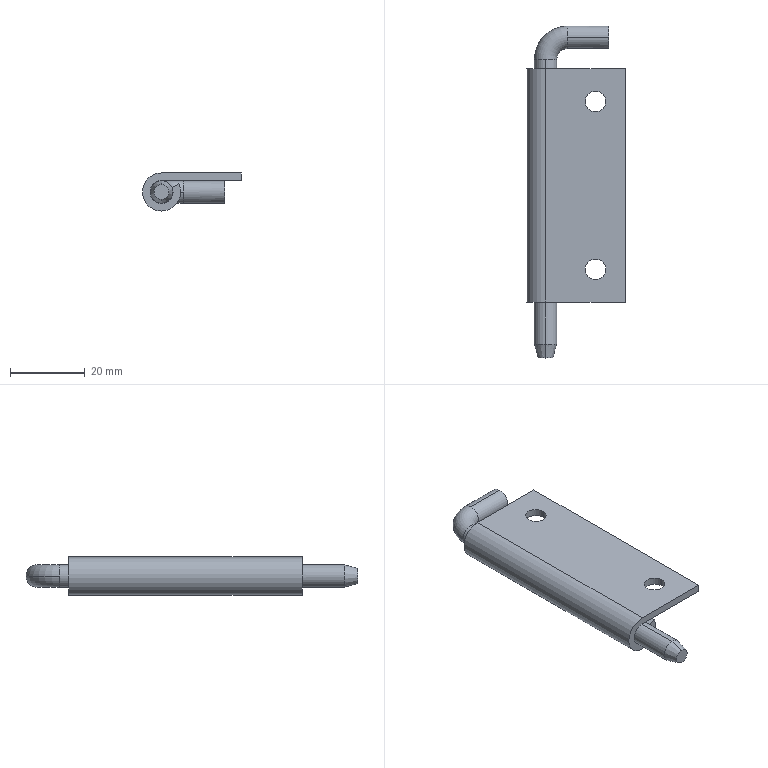Part | SolidWorks | features ICE 2, Chamfer 1, Sweep 1 | 2 solids | 24 faces | box 26.5 x 89 x 10.2 mm | volume 8027 mm3 | cylinder 12 | plane 8 | torus 2 | cone 2 | commonest cylinder face diameters 5.5 x4 6 x4 6.2 x2 10.2 x2
STEP:
#1=CARTESIAN_POINT('',(0.,80.,-3.));
#2=VERTEX_POINT('',#1);
#3=CARTESIAN_POINT('',(-3.,80.,0.));
#4=VERTEX_POINT('',#3);
#5=CARTESIAN_POINT('',(0.,80.,0.));
#6=DIRECTION('',(0.,1.,0.));
#7=DIRECTION('',(0.,0.,1.));
#8=AXIS2_PLACEMENT_3D('',#5,#6,#7);
#9=CIRCLE('',#8,3.);
#10=EDGE_CURVE('',#2,#4,#9,.T.);
#11=ORIENTED_EDGE('',*,*,#10,.T.);
#12=CARTESIAN_POINT('',(6.,89.,0.));
#13=VERTEX_POINT('',#12);
#14=CARTESIAN_POINT('',(6.,80.,0.));
#15=DIRECTION('',(0.,0.,-1.));
#16=DIRECTION('',(-1.,0.,0.));
#17=AXIS2_PLACEMENT_3D('',#14,#15,#16);
#18=CIRCLE('',#17,9.);
#19=EDGE_CURVE('',#4,#13,#18,.T.);
#20=ORIENTED_EDGE('',*,*,#19,.T.);
#21=CARTESIAN_POINT('',(6.,86.,-3.));
#22=VERTEX_POINT('',#21);
#23=CARTESIAN_POINT('',(6.,86.,0.));
#24=DIRECTION('',(1.,0.,0.));
#25=DIRECTION('',(0.,0.,1.));
#26=AXIS2_PLACEMENT_3D('',#23,#24,#25);
#27=CIRCLE('',#26,3.);
#28=EDGE_CURVE('',#22,#13,#27,.T.);
#29=ORIENTED_EDGE('',*,*,#28,.F.);
#30=CARTESIAN_POINT('',(6.,83.,0.));
#31=VERTEX_POINT('',#30);
#32=CARTESIAN_POINT('',(6.,86.,0.));
#33=DIRECTION('',(1.,0.,0.));
#34=DIRECTION('',(0.,0.,1.));
#35=AXIS2_PLACEMENT_3D('',#32,#33,#34);
#36=CIRCLE('',#35,3.);
#37=EDGE_CURVE('',#31,#22,#36,.T.);
#38=ORIENTED_EDGE('',*,*,#37,.F.);
#39=CARTESIAN_POINT('',(3.,80.,0.));
#40=VERTEX_POINT('',#39);
#41=CARTESIAN_POINT('',(6.,80.,0.));
#42=DIRECTION('',(0.,0.,-1.));
#43=DIRECTION('',(-1.,0.,0.));
#44=AXIS2_PLACEMENT_3D('',#41,#42,#43);
#45=CIRCLE('',#44,3.);
#46=EDGE_CURVE('',#40,#31,#45,.T.);
#47=ORIENTED_EDGE('',*,*,#46,.F.);
#48=CARTESIAN_POINT('',(0.,80.,0.));
#49=DIRECTION('',(0.,1.,0.));
#50=DIRECTION('',(0.,0.,1.));
#51=AXIS2_PLACEMENT_3D('',#48,#49,#50);
#52=CIRCLE('',#51,3.);
#53=EDGE_CURVE('',#40,#2,#52,.T.);
#54=ORIENTED_EDGE('',*,*,#53,.T.);
#55=EDGE_LOOP('',(#11,#20,#29,#38,#47,#54));
#56=FACE_OUTER_BOUND('',#55,.T.);
#57=CARTESIAN_POINT('',(6.,80.,0.));
#58=DIRECTION('',(0.,0.,-1.));
#59=DIRECTION('',(-1.,0.,0.));
#60=AXIS2_PLACEMENT_3D('',#57,#58,#59);
#61=TOROIDAL_SURFACE('',#60,6.,3.);
#62=ADVANCED_FACE('',(#56),#61,.T.);
#63=CARTESIAN_POINT('',(0.,0.,-2.));
#64=VERTEX_POINT('',#63);
#65=CARTESIAN_POINT('',(0.,0.,2.));
#66=VERTEX_POINT('',#65);
#67=CARTESIAN_POINT('',(0.,0.,0.));
#68=DIRECTION('',(0.,-1.,0.));
#69=DIRECTION('',(0.,0.,1.));
#70=AXIS2_PLACEMENT_3D('',#67,#68,#69);
#71=CIRCLE('',#70,2.);
#72=EDGE_CURVE('',#64,#66,#71,.T.);
#73=ORIENTED_EDGE('',*,*,#72,.F.);
#74=CARTESIAN_POINT('',(0.,3.732,-3.));
#75=VERTEX_POINT('',#74);
#76=CARTESIAN_POINT('',(0.,3.732,-3.));
#77=DIRECTION('',(0.,0.9659,-0.2588));
#78=VECTOR('',#77,1000.);
#79=LINE('',#76,#78);
#80=EDGE_CURVE('',#64,#75,#79,.T.);
#81=ORIENTED_EDGE('',*,*,#80,.T.);
#82=CARTESIAN_POINT('',(0.,3.732,3.));
#83=VERTEX_POINT('',#82);
#84=CARTESIAN_POINT('',(0.,3.732,0.));
#85=DIRECTION('',(0.,1.,0.));
#86=DIRECTION('',(0.,0.,1.));
#87=AXIS2_PLACEMENT_3D('',#84,#85,#86);
#88=CIRCLE('',#87,3.);
#89=EDGE_CURVE('',#83,#75,#88,.T.);
#90=ORIENTED_EDGE('',*,*,#89,.F.);
#91=CARTESIAN_POINT('',(0.,3.732,3.));
#92=DIRECTION('',(0.,0.9659,0.2588));
#93=VECTOR('',#92,1000.);
#94=LINE('',#91,#93);
#95=EDGE_CURVE('',#66,#83,#94,.T.);
#96=ORIENTED_EDGE('',*,*,#95,.F.);
#97=EDGE_LOOP('',(#73,#81,#90,#96));
#98=FACE_OUTER_BOUND('',#97,.T.);
#99=CARTESIAN_POINT('',(0.,3.732,0.));
#100=DIRECTION('',(0.,1.,0.));
#101=DIRECTION('',(0.,0.,1.));
#102=AXIS2_PLACEMENT_3D('',#99,#100,#101);
#103=CONICAL_SURFACE('',#102,3.,0.2618);
#104=ADVANCED_FACE('',(#98),#103,.T.);
#105=CARTESIAN_POINT('',(0.,80.,3.));
#106=VERTEX_POINT('',#105);
#107=CARTESIAN_POINT('',(0.,80.,0.));
#108=DIRECTION('',(0.,1.,0.));
#109=DIRECTION('',(0.,0.,1.));
#110=AXIS2_PLACEMENT_3D('',#107,#108,#109);
#111=CIRCLE('',#110,3.);
#112=EDGE_CURVE('',#106,#40,#111,.T.);
#113=ORIENTED_EDGE('',*,*,#112,.F.);
#114=CARTESIAN_POINT('',(0.,80.,3.));
#115=DIRECTION('',(0.,-1.,0.));
#116=VECTOR('',#115,1000.);
#117=LINE('',#114,#116);
#118=EDGE_CURVE('',#106,#83,#117,.T.);
#119=ORIENTED_EDGE('',*,*,#118,.T.);
#120=ORIENTED_EDGE('',*,*,#89,.T.);
#121=CARTESIAN_POINT('',(0.,80.,-3.));
#122=DIRECTION('',(0.,-1.,0.));
#123=VECTOR('',#122,1000.);
#124=LINE('',#121,#123);
#125=EDGE_CURVE('',#2,#75,#124,.T.);
#126=ORIENTED_EDGE('',*,*,#125,.F.);
#127=ORIENTED_EDGE('',*,*,#53,.F.);
#128=EDGE_LOOP('',(#113,#119,#120,#126,#127));
#129=FACE_OUTER_BOUND('',#128,.T.);
#130=CARTESIAN_POINT('',(0.,80.,0.));
#131=DIRECTION('',(0.,-1.,0.));
#132=DIRECTION('',(0.,0.,-1.));
#133=AXIS2_PLACEMENT_3D('',#130,#131,#132);
#134=CYLINDRICAL_SURFACE('',#133,3.);
#135=ADVANCED_FACE('',(#129),#134,.T.);
#136=ORIENTED_EDGE('',*,*,#28,.T.);
#137=CARTESIAN_POINT('',(6.,86.,3.));
#138=VERTEX_POINT('',#137);
#139=CARTESIAN_POINT('',(6.,86.,0.));
#140=DIRECTION('',(1.,0.,0.));
#141=DIRECTION('',(0.,0.,1.));
#142=AXIS2_PLACEMENT_3D('',#139,#140,#141);
#143=CIRCLE('',#142,3.);
#144=EDGE_CURVE('',#13,#138,#143,.T.);
#145=ORIENTED_EDGE('',*,*,#144,.T.);
#146=CARTESIAN_POINT('',(17.,86.,3.));
#147=VERTEX_POINT('',#146);
#148=CARTESIAN_POINT('',(6.,86.,3.));
#149=DIRECTION('',(1.,0.,0.));
#150=VECTOR('',#149,1000.);
#151=LINE('',#148,#150);
#152=EDGE_CURVE('',#138,#147,#151,.T.);
#153=ORIENTED_EDGE('',*,*,#152,.T.);
#154=CARTESIAN_POINT('',(17.,86.,-3.));
#155=VERTEX_POINT('',#154);
#156=CARTESIAN_POINT('',(17.,86.,0.));
#157=DIRECTION('',(1.,0.,0.));
#158=DIRECTION('',(0.,0.,1.));
#159=AXIS2_PLACEMENT_3D('',#156,#157,#158);
#160=CIRCLE('',#159,3.);
#161=EDGE_CURVE('',#155,#147,#160,.T.);
#162=ORIENTED_EDGE('',*,*,#161,.F.);
#163=CARTESIAN_POINT('',(6.,86.,-3.));
#164=DIRECTION('',(1.,0.,0.));
#165=VECTOR('',#164,1000.);
#166=LINE('',#163,#165);
#167=EDGE_CURVE('',#22,#155,#166,.T.);
#168=ORIENTED_EDGE('',*,*,#167,.F.);
#169=EDGE_LOOP('',(#136,#145,#153,#162,#168));
#170=FACE_OUTER_BOUND('',#169,.T.);
#171=CARTESIAN_POINT('',(6.,86.,0.));
#172=DIRECTION('',(1.,0.,0.));
#173=DIRECTION('',(0.,0.,-1.));
#174=AXIS2_PLACEMENT_3D('',#171,#172,#173);
#175=CYLINDRICAL_SURFACE('',#174,3.);
#176=ADVANCED_FACE('',(#170),#175,.T.);
#177=ORIENTED_EDGE('',*,*,#152,.F.);
#178=CARTESIAN_POINT('',(6.,86.,0.));
#179=DIRECTION('',(1.,0.,0.));
#180=DIRECTION('',(0.,0.,1.));
#181=AXIS2_PLACEMENT_3D('',#178,#179,#180);
#182=CIRCLE('',#181,3.);
#183=EDGE_CURVE('',#138,#31,#182,.T.);
#184=ORIENTED_EDGE('',*,*,#183,.T.);
#185=ORIENTED_EDGE('',*,*,#37,.T.);
#186=ORIENTED_EDGE('',*,*,#167,.T.);
#187=CARTESIAN_POINT('',(17.,86.,0.));
#188=DIRECTION('',(1.,0.,0.));
#189=DIRECTION('',(0.,0.,1.));
#190=AXIS2_PLACEMENT_3D('',#187,#188,#189);
#191=CIRCLE('',#190,3.);
#192=EDGE_CURVE('',#147,#155,#191,.T.);
#193=ORIENTED_EDGE('',*,*,#192,.F.);
#194=EDGE_LOOP('',(#177,#184,#185,#186,#193));
#195=FACE_OUTER_BOUND('',#194,.T.);
#196=CARTESIAN_POINT('',(6.,86.,0.));
#197=DIRECTION('',(1.,0.,0.));
#198=DIRECTION('',(0.,0.,-1.));
#199=AXIS2_PLACEMENT_3D('',#196,#197,#198);
#200=CYLINDRICAL_SURFACE('',#199,3.);
#201=ADVANCED_FACE('',(#195),#200,.T.);
#202=ORIENTED_EDGE('',*,*,#19,.F.);
#203=CARTESIAN_POINT('',(0.,80.,0.));
#204=DIRECTION('',(0.,1.,0.));
#205=DIRECTION('',(0.,0.,1.));
#206=AXIS2_PLACEMENT_3D('',#203,#204,#205);
#207=CIRCLE('',#206,3.);
#208=EDGE_CURVE('',#4,#106,#207,.T.);
#209=ORIENTED_EDGE('',*,*,#208,.T.);
#210=ORIENTED_EDGE('',*,*,#112,.T.);
#211=ORIENTED_EDGE('',*,*,#46,.T.);
#212=ORIENTED_EDGE('',*,*,#183,.F.);
#213=ORIENTED_EDGE('',*,*,#144,.F.);
#214=EDGE_LOOP('',(#202,#209,#210,#211,#212,#213));
#215=FACE_OUTER_BOUND('',#214,.T.);
#216=CARTESIAN_POINT('',(6.,80.,0.));
#217=DIRECTION('',(0.,0.,-1.));
#218=DIRECTION('',(-1.,0.,0.));
#219=AXIS2_PLACEMENT_3D('',#216,#217,#218);
#220=TOROIDAL_SURFACE('',#219,6.,3.);
#221=ADVANCED_FACE('',(#215),#220,.T.);
#222=ORIENTED_EDGE('',*,*,#118,.F.);
#223=ORIENTED_EDGE('',*,*,#208,.F.);
#224=ORIENTED_EDGE('',*,*,#10,.F.);
#225=ORIENTED_EDGE('',*,*,#125,.T.);
#226=CARTESIAN_POINT('',(0.,3.732,0.));
#227=DIRECTION('',(0.,1.,0.));
#228=DIRECTION('',(0.,0.,1.));
#229=AXIS2_PLACEMENT_3D('',#226,#227,#228);
#230=CIRCLE('',#229,3.);
#231=EDGE_CURVE('',#75,#83,#230,.T.);
#232=ORIENTED_EDGE('',*,*,#231,.T.);
#233=EDGE_LOOP('',(#222,#223,#224,#225,#232));
#234=FACE_OUTER_BOUND('',#233,.T.);
#235=CARTESIAN_POINT('',(0.,80.,0.));
#236=DIRECTION('',(0.,-1.,0.));
#237=DIRECTION('',(0.,0.,-1.));
#238=AXIS2_PLACEMENT_3D('',#235,#236,#237);
#239=CYLINDRICAL_SURFACE('',#238,3.);
#240=ADVANCED_FACE('',(#234),#239,.T.);
#241=ORIENTED_EDGE('',*,*,#161,.T.);
#242=ORIENTED_EDGE('',*,*,#192,.T.);
#243=EDGE_LOOP('',(#241,#242));
#244=FACE_OUTER_BOUND('',#243,.T.);
#245=CARTESIAN_POINT('',(17.,86.,0.));
#246=DIRECTION('',(1.,0.,0.));
#247=DIRECTION('',(0.,0.,1.));
#248=AXIS2_PLACEMENT_3D('',#245,#246,#247);
#249=PLANE('',#248);
#250=ADVANCED_FACE('',(#244),#249,.T.);
#251=CARTESIAN_POINT('',(0.,0.,0.));
#252=DIRECTION('',(0.,-1.,0.));
#253=DIRECTION('',(0.,0.,1.));
#254=AXIS2_PLACEMENT_3D('',#251,#252,#253);
#255=CIRCLE('',#254,2.);
#256=EDGE_CURVE('',#66,#64,#255,.T.);
#257=ORIENTED_EDGE('',*,*,#256,.T.);
#258=ORIENTED_EDGE('',*,*,#72,.T.);
#259=EDGE_LOOP('',(#257,#258));
#260=FACE_OUTER_BOUND('',#259,.T.);
#261=CARTESIAN_POINT('',(0.,0.,0.));
#262=DIRECTION('',(0.,1.,0.));
#263=DIRECTION('',(0.,0.,1.));
#264=AXIS2_PLACEMENT_3D('',#261,#262,#263);
#265=PLANE('',#264);
#266=ADVANCED_FACE('',(#260),#265,.F.);
#267=ORIENTED_EDGE('',*,*,#80,.F.);
#268=ORIENTED_EDGE('',*,*,#256,.F.);
#269=ORIENTED_EDGE('',*,*,#95,.T.);
#270=ORIENTED_EDGE('',*,*,#231,.F.);
#271=EDGE_LOOP('',(#267,#268,#269,#270));
#272=FACE_OUTER_BOUND('',#271,.T.);
#273=CARTESIAN_POINT('',(0.,3.732,0.));
#274=DIRECTION('',(0.,1.,0.));
#275=DIRECTION('',(0.,0.,1.));
#276=AXIS2_PLACEMENT_3D('',#273,#274,#275);
#277=CONICAL_SURFACE('',#276,3.,0.2618);
#278=ADVANCED_FACE('',(#272),#277,.T.);
#279=CLOSED_SHELL('',(#62,#104,#135,#176,#201,#221,#240,#250,#266,#278));
#280=MANIFOLD_SOLID_BREP('',#279);
#281=CARTESIAN_POINT('',(10.65,68.75,5.1));
#282=VERTEX_POINT('',#281);
#283=CARTESIAN_POINT('',(16.15,68.75,5.1));
#284=VERTEX_POINT('',#283);
#285=CARTESIAN_POINT('',(13.4,68.75,5.1));
#286=DIRECTION('',(0.,0.,1.));
#287=DIRECTION('',(1.,0.,0.));
#288=AXIS2_PLACEMENT_3D('',#285,#286,#287);
#289=CIRCLE('',#288,2.75);
#290=EDGE_CURVE('',#282,#284,#289,.T.);
#291=ORIENTED_EDGE('',*,*,#290,.T.);
#292=CARTESIAN_POINT('',(16.15,68.75,3.1));
#293=VERTEX_POINT('',#292);
#294=CARTESIAN_POINT('',(16.15,68.75,5.1));
#295=DIRECTION('',(0.,0.,-1.));
#296=VECTOR('',#295,1000.);
#297=LINE('',#294,#296);
#298=EDGE_CURVE('',#284,#293,#297,.T.);
#299=ORIENTED_EDGE('',*,*,#298,.T.);
#300=CARTESIAN_POINT('',(10.65,68.75,3.1));
#301=VERTEX_POINT('',#300);
#302=CARTESIAN_POINT('',(13.4,68.75,3.1));
#303=DIRECTION('',(0.,0.,1.));
#304=DIRECTION('',(1.,0.,0.));
#305=AXIS2_PLACEMENT_3D('',#302,#303,#304);
#306=CIRCLE('',#305,2.75);
#307=EDGE_CURVE('',#301,#293,#306,.T.);
#308=ORIENTED_EDGE('',*,*,#307,.F.);
#309=CARTESIAN_POINT('',(10.65,68.75,5.1));
#310=DIRECTION('',(0.,0.,-1.));
#311=VECTOR('',#310,1000.);
#312=LINE('',#309,#311);
#313=EDGE_CURVE('',#282,#301,#312,.T.);
#314=ORIENTED_EDGE('',*,*,#313,.F.);
#315=EDGE_LOOP('',(#291,#299,#308,#314));
#316=FACE_OUTER_BOUND('',#315,.T.);
#317=CARTESIAN_POINT('',(13.4,68.75,5.1));
#318=DIRECTION('',(0.,0.,-1.));
#319=DIRECTION('',(-1.,0.,0.));
#320=AXIS2_PLACEMENT_3D('',#317,#318,#319);
#321=CYLINDRICAL_SURFACE('',#320,2.75);
#322=ADVANCED_FACE('',(#316),#321,.F.);
#323=CARTESIAN_POINT('',(10.65,23.75,5.1));
#324=VERTEX_POINT('',#323);
#325=CARTESIAN_POINT('',(16.15,23.75,5.1));
#326=VERTEX_POINT('',#325);
#327=CARTESIAN_POINT('',(13.4,23.75,5.1));
#328=DIRECTION('',(0.,0.,1.));
#329=DIRECTION('',(1.,0.,0.));
#330=AXIS2_PLACEMENT_3D('',#327,#328,#329);
#331=CIRCLE('',#330,2.75);
#332=EDGE_CURVE('',#324,#326,#331,.T.);
#333=ORIENTED_EDGE('',*,*,#332,.T.);
#334=CARTESIAN_POINT('',(16.15,23.75,3.1));
#335=VERTEX_POINT('',#334);
#336=CARTESIAN_POINT('',(16.15,23.75,5.1));
#337=DIRECTION('',(0.,0.,-1.));
#338=VECTOR('',#337,1000.);
#339=LINE('',#336,#338);
#340=EDGE_CURVE('',#326,#335,#339,.T.);
#341=ORIENTED_EDGE('',*,*,#340,.T.);
#342=CARTESIAN_POINT('',(10.65,23.75,3.1));
#343=VERTEX_POINT('',#342);
#344=CARTESIAN_POINT('',(13.4,23.75,3.1));
#345=DIRECTION('',(0.,0.,1.));
#346=DIRECTION('',(1.,0.,0.));
#347=AXIS2_PLACEMENT_3D('',#344,#345,#346);
#348=CIRCLE('',#347,2.75);
#349=EDGE_CURVE('',#343,#335,#348,.T.);
#350=ORIENTED_EDGE('',*,*,#349,.F.);
#351=CARTESIAN_POINT('',(10.65,23.75,5.1));
#352=DIRECTION('',(0.,0.,-1.));
#353=VECTOR('',#352,1000.);
#354=LINE('',#351,#353);
#355=EDGE_CURVE('',#324,#343,#354,.T.);
#356=ORIENTED_EDGE('',*,*,#355,.F.);
#357=EDGE_LOOP('',(#333,#341,#350,#356));
#358=FACE_OUTER_BOUND('',#357,.T.);
#359=CARTESIAN_POINT('',(13.4,23.75,5.1));
#360=DIRECTION('',(0.,0.,-1.));
#361=DIRECTION('',(-1.,0.,0.));
#362=AXIS2_PLACEMENT_3D('',#359,#360,#361);
#363=CYLINDRICAL_SURFACE('',#362,2.75);
#364=ADVANCED_FACE('',(#358),#363,.F.);
#365=CARTESIAN_POINT('',(2.81,77.5,1.31));
#366=VERTEX_POINT('',#365);
#367=CARTESIAN_POINT('',(0.,77.5,-3.1));
#368=VERTEX_POINT('',#367);
#369=CARTESIAN_POINT('',(0.,77.5,0.));
#370=DIRECTION('',(0.,1.,0.));
#371=DIRECTION('',(0.,0.,1.));
#372=AXIS2_PLACEMENT_3D('',#369,#370,#371);
#373=CIRCLE('',#372,3.1);
#374=EDGE_CURVE('',#366,#368,#373,.T.);
#375=ORIENTED_EDGE('',*,*,#374,.T.);
#376=CARTESIAN_POINT('',(0.,15.,-3.1));
#377=VERTEX_POINT('',#376);
#378=CARTESIAN_POINT('',(0.,77.5,-3.1));
#379=DIRECTION('',(0.,-1.,0.));
#380=VECTOR('',#379,1000.);
#381=LINE('',#378,#380);
#382=EDGE_CURVE('',#368,#377,#381,.T.);
#383=ORIENTED_EDGE('',*,*,#382,.T.);
#384=CARTESIAN_POINT('',(2.81,15.,1.31));
#385=VERTEX_POINT('',#384);
#386=CARTESIAN_POINT('',(0.,15.,0.));
#387=DIRECTION('',(0.,1.,0.));
#388=DIRECTION('',(0.,0.,1.));
#389=AXIS2_PLACEMENT_3D('',#386,#387,#388);
#390=CIRCLE('',#389,3.1);
#391=EDGE_CURVE('',#385,#377,#390,.T.);
#392=ORIENTED_EDGE('',*,*,#391,.F.);
#393=CARTESIAN_POINT('',(2.81,77.5,1.31));
#394=DIRECTION('',(0.,-1.,0.));
#395=VECTOR('',#394,1000.);
#396=LINE('',#393,#395);
#397=EDGE_CURVE('',#366,#385,#396,.T.);
#398=ORIENTED_EDGE('',*,*,#397,.F.);
#399=EDGE_LOOP('',(#375,#383,#392,#398));
#400=FACE_OUTER_BOUND('',#399,.T.);
#401=CARTESIAN_POINT('',(0.,77.5,0.));
#402=DIRECTION('',(0.,-1.,0.));
#403=DIRECTION('',(0.,0.,-1.));
#404=AXIS2_PLACEMENT_3D('',#401,#402,#403);
#405=CYLINDRICAL_SURFACE('',#404,3.1);
#406=ADVANCED_FACE('',(#400),#405,.F.);
#407=CARTESIAN_POINT('',(0.,77.5,5.1));
#408=VERTEX_POINT('',#407);
#409=CARTESIAN_POINT('',(0.,77.5,-5.1));
#410=VERTEX_POINT('',#409);
#411=CARTESIAN_POINT('',(0.,77.5,0.));
#412=DIRECTION('',(0.,-1.,0.));
#413=DIRECTION('',(0.,0.,1.));
#414=AXIS2_PLACEMENT_3D('',#411,#412,#413);
#415=CIRCLE('',#414,5.1);
#416=EDGE_CURVE('',#408,#410,#415,.T.);
#417=ORIENTED_EDGE('',*,*,#416,.T.);
#418=CARTESIAN_POINT('',(0.,15.,-5.1));
#419=VERTEX_POINT('',#418);
#420=CARTESIAN_POINT('',(0.,77.5,-5.1));
#421=DIRECTION('',(0.,-1.,0.));
#422=VECTOR('',#421,1000.);
#423=LINE('',#420,#422);
#424=EDGE_CURVE('',#410,#419,#423,.T.);
#425=ORIENTED_EDGE('',*,*,#424,.T.);
#426=CARTESIAN_POINT('',(0.,15.,5.1));
#427=VERTEX_POINT('',#426);
#428=CARTESIAN_POINT('',(0.,15.,0.));
#429=DIRECTION('',(0.,-1.,0.));
#430=DIRECTION('',(0.,0.,1.));
#431=AXIS2_PLACEMENT_3D('',#428,#429,#430);
#432=CIRCLE('',#431,5.1);
#433=EDGE_CURVE('',#427,#419,#432,.T.);
#434=ORIENTED_EDGE('',*,*,#433,.F.);
#435=CARTESIAN_POINT('',(0.,77.5,5.1));
#436=DIRECTION('',(0.,-1.,0.));
#437=VECTOR('',#436,1000.);
#438=LINE('',#435,#437);
#439=EDGE_CURVE('',#408,#427,#438,.T.);
#440=ORIENTED_EDGE('',*,*,#439,.F.);
#441=EDGE_LOOP('',(#417,#425,#434,#440));
#442=FACE_OUTER_BOUND('',#441,.T.);
#443=CARTESIAN_POINT('',(0.,77.5,0.));
#444=DIRECTION('',(0.,-1.,0.));
#445=DIRECTION('',(0.,0.,-1.));
#446=AXIS2_PLACEMENT_3D('',#443,#444,#445);
#447=CYLINDRICAL_SURFACE('',#446,5.1);
#448=ADVANCED_FACE('',(#442),#447,.T.);
#449=ORIENTED_EDGE('',*,*,#332,.F.);
#450=CARTESIAN_POINT('',(13.4,23.75,5.1));
#451=DIRECTION('',(0.,0.,1.));
#452=DIRECTION('',(1.,0.,0.));
#453=AXIS2_PLACEMENT_3D('',#450,#451,#452);
#454=CIRCLE('',#453,2.75);
#455=EDGE_CURVE('',#326,#324,#454,.T.);
#456=ORIENTED_EDGE('',*,*,#455,.F.);
#457=EDGE_LOOP('',(#449,#456));
#458=FACE_BOUND('',#457,.T.);
#459=CARTESIAN_POINT('',(21.4,15.,5.1));
#460=VERTEX_POINT('',#459);
#461=CARTESIAN_POINT('',(0.,15.,5.1));
#462=DIRECTION('',(-1.,0.,0.));
#463=VECTOR('',#462,1000.);
#464=LINE('',#461,#463);
#465=EDGE_CURVE('',#460,#427,#464,.T.);
#466=ORIENTED_EDGE('',*,*,#465,.F.);
#467=CARTESIAN_POINT('',(21.4,77.5,5.1));
#468=VERTEX_POINT('',#467);
#469=CARTESIAN_POINT('',(21.4,77.5,5.1));
#470=DIRECTION('',(0.,-1.,0.));
#471=VECTOR('',#470,1000.);
#472=LINE('',#469,#471);
#473=EDGE_CURVE('',#468,#460,#472,.T.);
#474=ORIENTED_EDGE('',*,*,#473,.F.);
#475=CARTESIAN_POINT('',(0.,77.5,5.1));
#476=DIRECTION('',(-1.,0.,0.));
#477=VECTOR('',#476,1000.);
#478=LINE('',#475,#477);
#479=EDGE_CURVE('',#468,#408,#478,.T.);
#480=ORIENTED_EDGE('',*,*,#479,.T.);
#481=ORIENTED_EDGE('',*,*,#439,.T.);
#482=EDGE_LOOP('',(#466,#474,#480,#481));
#483=FACE_OUTER_BOUND('',#482,.T.);
#484=ORIENTED_EDGE('',*,*,#290,.F.);
#485=CARTESIAN_POINT('',(13.4,68.75,5.1));
#486=DIRECTION('',(0.,0.,1.));
#487=DIRECTION('',(1.,0.,0.));
#488=AXIS2_PLACEMENT_3D('',#485,#486,#487);
#489=CIRCLE('',#488,2.75);
#490=EDGE_CURVE('',#284,#282,#489,.T.);
#491=ORIENTED_EDGE('',*,*,#490,.F.);
#492=EDGE_LOOP('',(#484,#491));
#493=FACE_BOUND('',#492,.T.);
#494=CARTESIAN_POINT('',(0.,77.5,5.1));
#495=DIRECTION('',(0.,0.,1.));
#496=DIRECTION('',(1.,0.,0.));
#497=AXIS2_PLACEMENT_3D('',#494,#495,#496);
#498=PLANE('',#497);
#499=ADVANCED_FACE('',(#458,#483,#493),#498,.T.);
#500=ORIENTED_EDGE('',*,*,#349,.T.);
#501=CARTESIAN_POINT('',(13.4,23.75,3.1));
#502=DIRECTION('',(0.,0.,1.));
#503=DIRECTION('',(1.,0.,0.));
#504=AXIS2_PLACEMENT_3D('',#501,#502,#503);
#505=CIRCLE('',#504,2.75);
#506=EDGE_CURVE('',#335,#343,#505,.T.);
#507=ORIENTED_EDGE('',*,*,#506,.T.);
#508=EDGE_LOOP('',(#500,#507));
#509=FACE_BOUND('',#508,.T.);
#510=CARTESIAN_POINT('',(0.,15.,3.1));
#511=VERTEX_POINT('',#510);
#512=CARTESIAN_POINT('',(21.4,15.,3.1));
#513=VERTEX_POINT('',#512);
#514=CARTESIAN_POINT('',(0.,15.,3.1));
#515=DIRECTION('',(1.,0.,0.));
#516=VECTOR('',#515,1000.);
#517=LINE('',#514,#516);
#518=EDGE_CURVE('',#511,#513,#517,.T.);
#519=ORIENTED_EDGE('',*,*,#518,.F.);
#520=CARTESIAN_POINT('',(0.,77.5,3.1));
#521=VERTEX_POINT('',#520);
#522=CARTESIAN_POINT('',(0.,77.5,3.1));
#523=DIRECTION('',(0.,-1.,0.));
#524=VECTOR('',#523,1000.);
#525=LINE('',#522,#524);
#526=EDGE_CURVE('',#521,#511,#525,.T.);
#527=ORIENTED_EDGE('',*,*,#526,.F.);
#528=CARTESIAN_POINT('',(21.4,77.5,3.1));
#529=VERTEX_POINT('',#528);
#530=CARTESIAN_POINT('',(0.,77.5,3.1));
#531=DIRECTION('',(1.,0.,0.));
#532=VECTOR('',#531,1000.);
#533=LINE('',#530,#532);
#534=EDGE_CURVE('',#521,#529,#533,.T.);
#535=ORIENTED_EDGE('',*,*,#534,.T.);
#536=CARTESIAN_POINT('',(21.4,77.5,3.1));
#537=DIRECTION('',(0.,-1.,0.));
#538=VECTOR('',#537,1000.);
#539=LINE('',#536,#538);
#540=EDGE_CURVE('',#529,#513,#539,.T.);
#541=ORIENTED_EDGE('',*,*,#540,.T.);
#542=EDGE_LOOP('',(#519,#527,#535,#541));
#543=FACE_OUTER_BOUND('',#542,.T.);
#544=ORIENTED_EDGE('',*,*,#307,.T.);
#545=CARTESIAN_POINT('',(13.4,68.75,3.1));
#546=DIRECTION('',(0.,0.,1.));
#547=DIRECTION('',(1.,0.,0.));
#548=AXIS2_PLACEMENT_3D('',#545,#546,#547);
#549=CIRCLE('',#548,2.75);
#550=EDGE_CURVE('',#293,#301,#549,.T.);
#551=ORIENTED_EDGE('',*,*,#550,.T.);
#552=EDGE_LOOP('',(#544,#551));
#553=FACE_BOUND('',#552,.T.);
#554=CARTESIAN_POINT('',(0.,77.5,3.1));
#555=DIRECTION('',(0.,0.,-1.));
#556=DIRECTION('',(-1.,0.,0.));
#557=AXIS2_PLACEMENT_3D('',#554,#555,#556);
#558=PLANE('',#557);
#559=ADVANCED_FACE('',(#509,#543,#553),#558,.T.);
#560=ORIENTED_EDGE('',*,*,#424,.F.);
#561=CARTESIAN_POINT('',(4.622,77.5,2.155));
#562=VERTEX_POINT('',#561);
#563=CARTESIAN_POINT('',(0.,77.5,0.));
#564=DIRECTION('',(0.,-1.,0.));
#565=DIRECTION('',(0.,0.,1.));
#566=AXIS2_PLACEMENT_3D('',#563,#564,#565);
#567=CIRCLE('',#566,5.1);
#568=EDGE_CURVE('',#410,#562,#567,.T.);
#569=ORIENTED_EDGE('',*,*,#568,.T.);
#570=CARTESIAN_POINT('',(4.622,15.,2.155));
#571=VERTEX_POINT('',#570);
#572=CARTESIAN_POINT('',(4.622,77.5,2.155));
#573=DIRECTION('',(0.,-1.,0.));
#574=VECTOR('',#573,1000.);
#575=LINE('',#572,#574);
#576=EDGE_CURVE('',#562,#571,#575,.T.);
#577=ORIENTED_EDGE('',*,*,#576,.T.);
#578=CARTESIAN_POINT('',(0.,15.,0.));
#579=DIRECTION('',(0.,-1.,0.));
#580=DIRECTION('',(0.,0.,1.));
#581=AXIS2_PLACEMENT_3D('',#578,#579,#580);
#582=CIRCLE('',#581,5.1);
#583=EDGE_CURVE('',#419,#571,#582,.T.);
#584=ORIENTED_EDGE('',*,*,#583,.F.);
#585=EDGE_LOOP('',(#560,#569,#577,#584));
#586=FACE_OUTER_BOUND('',#585,.T.);
#587=CARTESIAN_POINT('',(0.,77.5,0.));
#588=DIRECTION('',(0.,-1.,0.));
#589=DIRECTION('',(0.,0.,-1.));
#590=AXIS2_PLACEMENT_3D('',#587,#588,#589);
#591=CYLINDRICAL_SURFACE('',#590,5.1);
#592=ADVANCED_FACE('',(#586),#591,.T.);
#593=CARTESIAN_POINT('',(21.4,15.,3.1));
#594=DIRECTION('',(0.,0.,1.));
#595=VECTOR('',#594,1000.);
#596=LINE('',#593,#595);
#597=EDGE_CURVE('',#513,#460,#596,.T.);
#598=ORIENTED_EDGE('',*,*,#597,.F.);
#599=ORIENTED_EDGE('',*,*,#540,.F.);
#600=CARTESIAN_POINT('',(21.4,77.5,3.1));
#601=DIRECTION('',(0.,0.,1.));
#602=VECTOR('',#601,1000.);
#603=LINE('',#600,#602);
#604=EDGE_CURVE('',#529,#468,#603,.T.);
#605=ORIENTED_EDGE('',*,*,#604,.T.);
#606=ORIENTED_EDGE('',*,*,#473,.T.);
#607=EDGE_LOOP('',(#598,#599,#605,#606));
#608=FACE_OUTER_BOUND('',#607,.T.);
#609=CARTESIAN_POINT('',(21.4,77.5,3.1));
#610=DIRECTION('',(1.,0.,0.));
#611=DIRECTION('',(0.,0.,-1.));
#612=AXIS2_PLACEMENT_3D('',#609,#610,#611);
#613=PLANE('',#612);
#614=ADVANCED_FACE('',(#608),#613,.T.);
#615=ORIENTED_EDGE('',*,*,#382,.F.);
#616=CARTESIAN_POINT('',(0.,77.5,0.));
#617=DIRECTION('',(0.,1.,0.));
#618=DIRECTION('',(0.,0.,1.));
#619=AXIS2_PLACEMENT_3D('',#616,#617,#618);
#620=CIRCLE('',#619,3.1);
#621=EDGE_CURVE('',#368,#521,#620,.T.);
#622=ORIENTED_EDGE('',*,*,#621,.T.);
#623=ORIENTED_EDGE('',*,*,#526,.T.);
#624=CARTESIAN_POINT('',(0.,15.,0.));
#625=DIRECTION('',(0.,1.,0.));
#626=DIRECTION('',(0.,0.,1.));
#627=AXIS2_PLACEMENT_3D('',#624,#625,#626);
#628=CIRCLE('',#627,3.1);
#629=EDGE_CURVE('',#377,#511,#628,.T.);
#630=ORIENTED_EDGE('',*,*,#629,.F.);
#631=EDGE_LOOP('',(#615,#622,#623,#630));
#632=FACE_OUTER_BOUND('',#631,.T.);
#633=CARTESIAN_POINT('',(0.,77.5,0.));
#634=DIRECTION('',(0.,-1.,0.));
#635=DIRECTION('',(0.,0.,-1.));
#636=AXIS2_PLACEMENT_3D('',#633,#634,#635);
#637=CYLINDRICAL_SURFACE('',#636,3.1);
#638=ADVANCED_FACE('',(#632),#637,.F.);
#639=CARTESIAN_POINT('',(2.81,15.,1.31));
#640=DIRECTION('',(-0.9063,0.,-0.4226));
#641=VECTOR('',#640,1000.);
#642=LINE('',#639,#641);
#643=EDGE_CURVE('',#571,#385,#642,.T.);
#644=ORIENTED_EDGE('',*,*,#643,.F.);
#645=ORIENTED_EDGE('',*,*,#576,.F.);
#646=CARTESIAN_POINT('',(2.81,77.5,1.31));
#647=DIRECTION('',(-0.9063,0.,-0.4226));
#648=VECTOR('',#647,1000.);
#649=LINE('',#646,#648);
#650=EDGE_CURVE('',#562,#366,#649,.T.);
#651=ORIENTED_EDGE('',*,*,#650,.T.);
#652=ORIENTED_EDGE('',*,*,#397,.T.);
#653=EDGE_LOOP('',(#644,#645,#651,#652));
#654=FACE_OUTER_BOUND('',#653,.T.);
#655=CARTESIAN_POINT('',(2.81,77.5,1.31));
#656=DIRECTION('',(-0.4226,0.,0.9063));
#657=DIRECTION('',(0.9063,0.,0.4226));
#658=AXIS2_PLACEMENT_3D('',#655,#656,#657);
#659=PLANE('',#658);
#660=ADVANCED_FACE('',(#654),#659,.T.);
#661=ORIENTED_EDGE('',*,*,#416,.F.);
#662=ORIENTED_EDGE('',*,*,#479,.F.);
#663=ORIENTED_EDGE('',*,*,#604,.F.);
#664=ORIENTED_EDGE('',*,*,#534,.F.);
#665=ORIENTED_EDGE('',*,*,#621,.F.);
#666=ORIENTED_EDGE('',*,*,#374,.F.);
#667=ORIENTED_EDGE('',*,*,#650,.F.);
#668=ORIENTED_EDGE('',*,*,#568,.F.);
#669=EDGE_LOOP('',(#661,#662,#663,#664,#665,#666,#667,#668));
#670=FACE_OUTER_BOUND('',#669,.T.);
#671=CARTESIAN_POINT('',(0.,77.5,0.));
#672=DIRECTION('',(0.,1.,0.));
#673=DIRECTION('',(0.,0.,1.));
#674=AXIS2_PLACEMENT_3D('',#671,#672,#673);
#675=PLANE('',#674);
#676=ADVANCED_FACE('',(#670),#675,.T.);
#677=ORIENTED_EDGE('',*,*,#433,.T.);
#678=ORIENTED_EDGE('',*,*,#583,.T.);
#679=ORIENTED_EDGE('',*,*,#643,.T.);
#680=ORIENTED_EDGE('',*,*,#391,.T.);
#681=ORIENTED_EDGE('',*,*,#629,.T.);
#682=ORIENTED_EDGE('',*,*,#518,.T.);
#683=ORIENTED_EDGE('',*,*,#597,.T.);
#684=ORIENTED_EDGE('',*,*,#465,.T.);
#685=EDGE_LOOP('',(#677,#678,#679,#680,#681,#682,#683,#684));
#686=FACE_OUTER_BOUND('',#685,.T.);
#687=CARTESIAN_POINT('',(0.,15.,0.));
#688=DIRECTION('',(0.,1.,0.));
#689=DIRECTION('',(0.,0.,1.));
#690=AXIS2_PLACEMENT_3D('',#687,#688,#689);
#691=PLANE('',#690);
#692=ADVANCED_FACE('',(#686),#691,.F.);
#693=ORIENTED_EDGE('',*,*,#340,.F.);
#694=ORIENTED_EDGE('',*,*,#455,.T.);
#695=ORIENTED_EDGE('',*,*,#355,.T.);
#696=ORIENTED_EDGE('',*,*,#506,.F.);
#697=EDGE_LOOP('',(#693,#694,#695,#696));
#698=FACE_OUTER_BOUND('',#697,.T.);
#699=CARTESIAN_POINT('',(13.4,23.75,5.1));
#700=DIRECTION('',(0.,0.,-1.));
#701=DIRECTION('',(-1.,0.,0.));
#702=AXIS2_PLACEMENT_3D('',#699,#700,#701);
#703=CYLINDRICAL_SURFACE('',#702,2.75);
#704=ADVANCED_FACE('',(#698),#703,.F.);
#705=ORIENTED_EDGE('',*,*,#298,.F.);
#706=ORIENTED_EDGE('',*,*,#490,.T.);
#707=ORIENTED_EDGE('',*,*,#313,.T.);
#708=ORIENTED_EDGE('',*,*,#550,.F.);
#709=EDGE_LOOP('',(#705,#706,#707,#708));
#710=FACE_OUTER_BOUND('',#709,.T.);
#711=CARTESIAN_POINT('',(13.4,68.75,5.1));
#712=DIRECTION('',(0.,0.,-1.));
#713=DIRECTION('',(-1.,0.,0.));
#714=AXIS2_PLACEMENT_3D('',#711,#712,#713);
#715=CYLINDRICAL_SURFACE('',#714,2.75);
#716=ADVANCED_FACE('',(#710),#715,.F.);
#717=CLOSED_SHELL('',(#322,#364,#406,#448,#499,#559,#592,#614,#638,#660,#676,#692,#704,#716));
#718=MANIFOLD_SOLID_BREP('',#717);
#719=CARTESIAN_POINT('',(0.,0.,0.));
#720=DIRECTION('',(0.,0.,1.));
#721=DIRECTION('',(1.,0.,0.));
#722=AXIS2_PLACEMENT_3D('',#719,#720,#721);
#723=(LENGTH_UNIT()NAMED_UNIT(*)SI_UNIT(.MILLI.,.METRE.));
#724=UNCERTAINTY_MEASURE_WITH_UNIT(LENGTH_MEASURE(0.00001),#723,'','');
#725=(NAMED_UNIT(*)PLANE_ANGLE_UNIT()SI_UNIT($,.RADIAN.));
#726=(NAMED_UNIT(*)SI_UNIT($,.STERADIAN.)SOLID_ANGLE_UNIT());
#727=(GEOMETRIC_REPRESENTATION_CONTEXT(3)GLOBAL_UNCERTAINTY_ASSIGNED_CONTEXT((#724))GLOBAL_UNIT_ASSIGNED_CONTEXT((#723,#725,#726))REPRESENTATION_CONTEXT('',''));
#728=ADVANCED_BREP_SHAPE_REPRESENTATION('',(#280,#718,#722),#727);